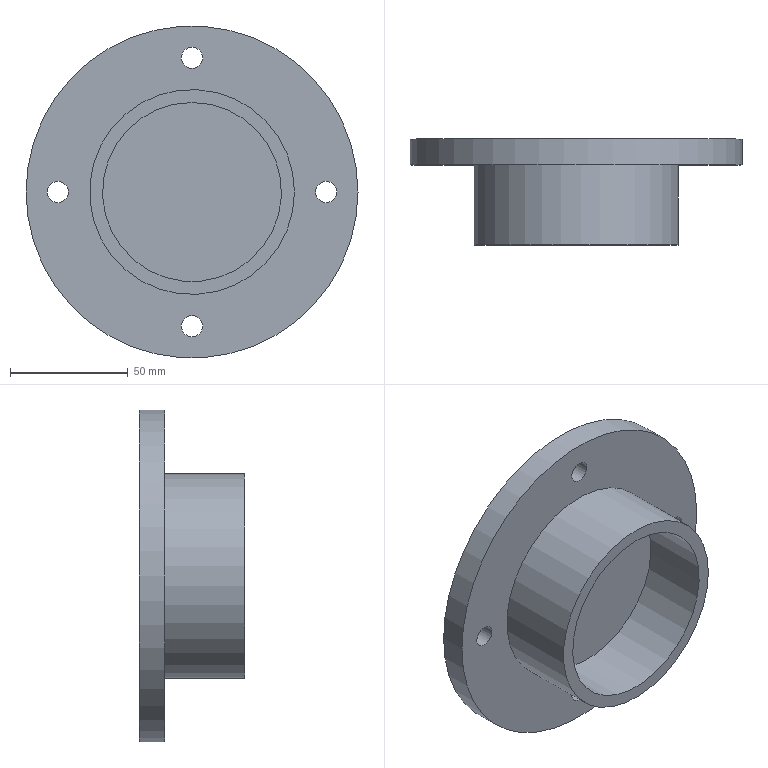Part | NX | features DATUM_CSYS 7, HOLE PACKAGE 7, SIMPLE HOLE 7, SKETCH 6, EXTRACT_DATUM_AXIS 4, EXTRACT_FACE 4, Instance Feature 3, EXTRUDE 2, DELETE FACE 1, Pattern Feature 1 | 1 solid | 13 faces | box 141 x 45 x 141 mm | volume 224063 mm3 | cylinder 8 | plane 5 | commonest cylinder face diameters 9 x4 76 x1 81 x1 87 x1 141 x1
STEP:
#1=CARTESIAN_POINT('',(70.5,-11.,0.));
#2=VERTEX_POINT('',#1);
#3=CARTESIAN_POINT('',(0.,-11.,0.));
#4=DIRECTION('',(0.,-1.,0.));
#5=DIRECTION('',(1.,0.,0.));
#6=AXIS2_PLACEMENT_3D('',#3,#4,#5);
#7=CIRCLE('',#6,70.5);
#8=EDGE_CURVE('',#2,#2,#7,.T.);
#9=ORIENTED_EDGE('',*,*,#8,.F.);
#10=EDGE_LOOP('',(#9));
#11=FACE_BOUND('',#10,.T.);
#12=CARTESIAN_POINT('',(70.5,0.,0.));
#13=VERTEX_POINT('',#12);
#14=CARTESIAN_POINT('',(0.,0.,0.));
#15=DIRECTION('',(0.,-1.,0.));
#16=DIRECTION('',(1.,0.,0.));
#17=AXIS2_PLACEMENT_3D('',#14,#15,#16);
#18=CIRCLE('',#17,70.5);
#19=EDGE_CURVE('',#13,#13,#18,.T.);
#20=ORIENTED_EDGE('',*,*,#19,.T.);
#21=EDGE_LOOP('',(#20));
#22=FACE_BOUND('',#21,.T.);
#23=CARTESIAN_POINT('',(0.,-11.,0.));
#24=DIRECTION('',(0.,1.,0.));
#25=DIRECTION('',(0.,0.,1.));
#26=AXIS2_PLACEMENT_3D('',#23,#24,#25);
#27=CYLINDRICAL_SURFACE('',#26,70.5);
#28=ADVANCED_FACE('',(#11,#22),#27,.T.);
#29=CARTESIAN_POINT('',(0.,-11.,-61.5));
#30=VERTEX_POINT('',#29);
#31=CARTESIAN_POINT('',(0.,-11.,-57.));
#32=DIRECTION('',(0.,-1.,0.));
#33=DIRECTION('',(0.,0.,-1.));
#34=AXIS2_PLACEMENT_3D('',#31,#32,#33);
#35=CIRCLE('',#34,4.5);
#36=EDGE_CURVE('',#30,#30,#35,.T.);
#37=ORIENTED_EDGE('',*,*,#36,.F.);
#38=EDGE_LOOP('',(#37));
#39=FACE_BOUND('',#38,.T.);
#40=CARTESIAN_POINT('',(57.,-11.,-4.5));
#41=VERTEX_POINT('',#40);
#42=CARTESIAN_POINT('',(57.,-11.,0.));
#43=DIRECTION('',(0.,-1.,0.));
#44=DIRECTION('',(0.,0.,-1.));
#45=AXIS2_PLACEMENT_3D('',#42,#43,#44);
#46=CIRCLE('',#45,4.5);
#47=EDGE_CURVE('',#41,#41,#46,.T.);
#48=ORIENTED_EDGE('',*,*,#47,.F.);
#49=EDGE_LOOP('',(#48));
#50=FACE_BOUND('',#49,.T.);
#51=CARTESIAN_POINT('',(0.,-11.,52.5));
#52=VERTEX_POINT('',#51);
#53=CARTESIAN_POINT('',(0.,-11.,57.));
#54=DIRECTION('',(0.,-1.,0.));
#55=DIRECTION('',(0.,0.,-1.));
#56=AXIS2_PLACEMENT_3D('',#53,#54,#55);
#57=CIRCLE('',#56,4.5);
#58=EDGE_CURVE('',#52,#52,#57,.T.);
#59=ORIENTED_EDGE('',*,*,#58,.F.);
#60=EDGE_LOOP('',(#59));
#61=FACE_BOUND('',#60,.T.);
#62=CARTESIAN_POINT('',(-57.,-11.,-4.5));
#63=VERTEX_POINT('',#62);
#64=CARTESIAN_POINT('',(-57.,-11.,0.));
#65=DIRECTION('',(0.,-1.,0.));
#66=DIRECTION('',(0.,0.,-1.));
#67=AXIS2_PLACEMENT_3D('',#64,#65,#66);
#68=CIRCLE('',#67,4.5);
#69=EDGE_CURVE('',#63,#63,#68,.T.);
#70=ORIENTED_EDGE('',*,*,#69,.F.);
#71=EDGE_LOOP('',(#70));
#72=FACE_BOUND('',#71,.T.);
#73=CARTESIAN_POINT('',(43.5,-11.,0.));
#74=VERTEX_POINT('',#73);
#75=CARTESIAN_POINT('',(0.,-11.,0.));
#76=DIRECTION('',(0.,-1.,0.));
#77=DIRECTION('',(1.,0.,0.));
#78=AXIS2_PLACEMENT_3D('',#75,#76,#77);
#79=CIRCLE('',#78,43.5);
#80=EDGE_CURVE('',#74,#74,#79,.T.);
#81=ORIENTED_EDGE('',*,*,#80,.F.);
#82=EDGE_LOOP('',(#81));
#83=FACE_BOUND('',#82,.T.);
#84=ORIENTED_EDGE('',*,*,#8,.T.);
#85=EDGE_LOOP('',(#84));
#86=FACE_BOUND('',#85,.T.);
#87=CARTESIAN_POINT('',(0.,-11.,0.));
#88=DIRECTION('',(0.,-1.,0.));
#89=DIRECTION('',(0.,0.,-1.));
#90=AXIS2_PLACEMENT_3D('',#87,#88,#89);
#91=PLANE('',#90);
#92=ADVANCED_FACE('',(#39,#50,#61,#72,#83,#86),#91,.T.);
#93=CARTESIAN_POINT('',(0.,0.,-61.5));
#94=VERTEX_POINT('',#93);
#95=CARTESIAN_POINT('',(0.,0.,-57.));
#96=DIRECTION('',(0.,-1.,0.));
#97=DIRECTION('',(0.,0.,-1.));
#98=AXIS2_PLACEMENT_3D('',#95,#96,#97);
#99=CIRCLE('',#98,4.5);
#100=EDGE_CURVE('',#94,#94,#99,.T.);
#101=ORIENTED_EDGE('',*,*,#100,.T.);
#102=EDGE_LOOP('',(#101));
#103=FACE_BOUND('',#102,.T.);
#104=CARTESIAN_POINT('',(57.,0.,-4.5));
#105=VERTEX_POINT('',#104);
#106=CARTESIAN_POINT('',(57.,0.,0.));
#107=DIRECTION('',(0.,-1.,0.));
#108=DIRECTION('',(0.,0.,-1.));
#109=AXIS2_PLACEMENT_3D('',#106,#107,#108);
#110=CIRCLE('',#109,4.5);
#111=EDGE_CURVE('',#105,#105,#110,.T.);
#112=ORIENTED_EDGE('',*,*,#111,.T.);
#113=EDGE_LOOP('',(#112));
#114=FACE_BOUND('',#113,.T.);
#115=CARTESIAN_POINT('',(0.,0.,52.5));
#116=VERTEX_POINT('',#115);
#117=CARTESIAN_POINT('',(0.,0.,57.));
#118=DIRECTION('',(0.,-1.,0.));
#119=DIRECTION('',(0.,0.,-1.));
#120=AXIS2_PLACEMENT_3D('',#117,#118,#119);
#121=CIRCLE('',#120,4.5);
#122=EDGE_CURVE('',#116,#116,#121,.T.);
#123=ORIENTED_EDGE('',*,*,#122,.T.);
#124=EDGE_LOOP('',(#123));
#125=FACE_BOUND('',#124,.T.);
#126=CARTESIAN_POINT('',(-57.,0.,-4.5));
#127=VERTEX_POINT('',#126);
#128=CARTESIAN_POINT('',(-57.,0.,0.));
#129=DIRECTION('',(0.,-1.,0.));
#130=DIRECTION('',(0.,0.,-1.));
#131=AXIS2_PLACEMENT_3D('',#128,#129,#130);
#132=CIRCLE('',#131,4.5);
#133=EDGE_CURVE('',#127,#127,#132,.T.);
#134=ORIENTED_EDGE('',*,*,#133,.T.);
#135=EDGE_LOOP('',(#134));
#136=FACE_BOUND('',#135,.T.);
#137=CARTESIAN_POINT('',(0.,0.,-40.5));
#138=VERTEX_POINT('',#137);
#139=CARTESIAN_POINT('',(0.,0.,0.));
#140=DIRECTION('',(0.,-1.,0.));
#141=DIRECTION('',(0.,0.,-1.));
#142=AXIS2_PLACEMENT_3D('',#139,#140,#141);
#143=CIRCLE('',#142,40.5);
#144=EDGE_CURVE('',#138,#138,#143,.T.);
#145=ORIENTED_EDGE('',*,*,#144,.T.);
#146=EDGE_LOOP('',(#145));
#147=FACE_BOUND('',#146,.T.);
#148=ORIENTED_EDGE('',*,*,#19,.F.);
#149=EDGE_LOOP('',(#148));
#150=FACE_BOUND('',#149,.T.);
#151=CARTESIAN_POINT('',(0.,0.,0.));
#152=DIRECTION('',(0.,-1.,0.));
#153=DIRECTION('',(0.,0.,-1.));
#154=AXIS2_PLACEMENT_3D('',#151,#152,#153);
#155=PLANE('',#154);
#156=ADVANCED_FACE('',(#103,#114,#125,#136,#147,#150),#155,.F.);
#157=CARTESIAN_POINT('',(43.5,-45.,0.));
#158=VERTEX_POINT('',#157);
#159=CARTESIAN_POINT('',(0.,-45.,0.));
#160=DIRECTION('',(0.,-1.,0.));
#161=DIRECTION('',(1.,0.,0.));
#162=AXIS2_PLACEMENT_3D('',#159,#160,#161);
#163=CIRCLE('',#162,43.5);
#164=EDGE_CURVE('',#158,#158,#163,.T.);
#165=ORIENTED_EDGE('',*,*,#164,.F.);
#166=EDGE_LOOP('',(#165));
#167=FACE_BOUND('',#166,.T.);
#168=ORIENTED_EDGE('',*,*,#80,.T.);
#169=EDGE_LOOP('',(#168));
#170=FACE_BOUND('',#169,.T.);
#171=CARTESIAN_POINT('',(0.,-45.,0.));
#172=DIRECTION('',(0.,1.,0.));
#173=DIRECTION('',(0.,0.,1.));
#174=AXIS2_PLACEMENT_3D('',#171,#172,#173);
#175=CYLINDRICAL_SURFACE('',#174,43.5);
#176=ADVANCED_FACE('',(#167,#170),#175,.T.);
#177=CARTESIAN_POINT('',(0.,-45.,38.));
#178=VERTEX_POINT('',#177);
#179=CARTESIAN_POINT('',(0.,-45.,0.));
#180=DIRECTION('',(0.,1.,0.));
#181=DIRECTION('',(0.,0.,1.));
#182=AXIS2_PLACEMENT_3D('',#179,#180,#181);
#183=CIRCLE('',#182,38.);
#184=EDGE_CURVE('',#178,#178,#183,.T.);
#185=ORIENTED_EDGE('',*,*,#184,.T.);
#186=EDGE_LOOP('',(#185));
#187=FACE_BOUND('',#186,.T.);
#188=ORIENTED_EDGE('',*,*,#164,.T.);
#189=EDGE_LOOP('',(#188));
#190=FACE_BOUND('',#189,.T.);
#191=CARTESIAN_POINT('',(0.,-45.,0.));
#192=DIRECTION('',(0.,-1.,0.));
#193=DIRECTION('',(0.,0.,-1.));
#194=AXIS2_PLACEMENT_3D('',#191,#192,#193);
#195=PLANE('',#194);
#196=ADVANCED_FACE('',(#187,#190),#195,.T.);
#197=CARTESIAN_POINT('',(0.,-16.,38.));
#198=VERTEX_POINT('',#197);
#199=CARTESIAN_POINT('',(0.,-16.,0.));
#200=DIRECTION('',(0.,1.,0.));
#201=DIRECTION('',(0.,0.,1.));
#202=AXIS2_PLACEMENT_3D('',#199,#200,#201);
#203=CIRCLE('',#202,38.);
#204=EDGE_CURVE('',#198,#198,#203,.F.);
#205=ORIENTED_EDGE('',*,*,#204,.T.);
#206=EDGE_LOOP('',(#205));
#207=FACE_BOUND('',#206,.T.);
#208=CARTESIAN_POINT('',(0.,-16.,0.));
#209=DIRECTION('',(0.,1.,0.));
#210=DIRECTION('',(0.,0.,1.));
#211=AXIS2_PLACEMENT_3D('',#208,#209,#210);
#212=PLANE('',#211);
#213=ADVANCED_FACE('',(#207),#212,.F.);
#214=ORIENTED_EDGE('',*,*,#204,.F.);
#215=EDGE_LOOP('',(#214));
#216=FACE_BOUND('',#215,.T.);
#217=ORIENTED_EDGE('',*,*,#184,.F.);
#218=EDGE_LOOP('',(#217));
#219=FACE_BOUND('',#218,.T.);
#220=CARTESIAN_POINT('',(0.,-45.,0.));
#221=DIRECTION('',(0.,1.,0.));
#222=DIRECTION('',(0.,0.,1.));
#223=AXIS2_PLACEMENT_3D('',#220,#221,#222);
#224=CYLINDRICAL_SURFACE('',#223,38.);
#225=ADVANCED_FACE('',(#216,#219),#224,.F.);
#226=CARTESIAN_POINT('',(0.,-3.,-40.5));
#227=VERTEX_POINT('',#226);
#228=CARTESIAN_POINT('',(0.,-3.,0.));
#229=DIRECTION('',(0.,-1.,0.));
#230=DIRECTION('',(0.,0.,-1.));
#231=AXIS2_PLACEMENT_3D('',#228,#229,#230);
#232=CIRCLE('',#231,40.5);
#233=EDGE_CURVE('',#227,#227,#232,.F.);
#234=ORIENTED_EDGE('',*,*,#233,.T.);
#235=EDGE_LOOP('',(#234));
#236=FACE_BOUND('',#235,.T.);
#237=CARTESIAN_POINT('',(0.,-3.,0.));
#238=DIRECTION('',(0.,-1.,0.));
#239=DIRECTION('',(0.,0.,-1.));
#240=AXIS2_PLACEMENT_3D('',#237,#238,#239);
#241=PLANE('',#240);
#242=ADVANCED_FACE('',(#236),#241,.F.);
#243=ORIENTED_EDGE('',*,*,#233,.F.);
#244=EDGE_LOOP('',(#243));
#245=FACE_BOUND('',#244,.T.);
#246=ORIENTED_EDGE('',*,*,#144,.F.);
#247=EDGE_LOOP('',(#246));
#248=FACE_BOUND('',#247,.T.);
#249=CARTESIAN_POINT('',(0.,0.,0.));
#250=DIRECTION('',(0.,-1.,0.));
#251=DIRECTION('',(0.,0.,-1.));
#252=AXIS2_PLACEMENT_3D('',#249,#250,#251);
#253=CYLINDRICAL_SURFACE('',#252,40.5);
#254=ADVANCED_FACE('',(#245,#248),#253,.F.);
#255=ORIENTED_EDGE('',*,*,#69,.T.);
#256=EDGE_LOOP('',(#255));
#257=FACE_BOUND('',#256,.T.);
#258=ORIENTED_EDGE('',*,*,#133,.F.);
#259=EDGE_LOOP('',(#258));
#260=FACE_BOUND('',#259,.T.);
#261=CARTESIAN_POINT('',(-57.,0.,0.));
#262=DIRECTION('',(0.,-1.,0.));
#263=DIRECTION('',(0.,0.,-1.));
#264=AXIS2_PLACEMENT_3D('',#261,#262,#263);
#265=CYLINDRICAL_SURFACE('',#264,4.5);
#266=ADVANCED_FACE('',(#257,#260),#265,.F.);
#267=ORIENTED_EDGE('',*,*,#58,.T.);
#268=EDGE_LOOP('',(#267));
#269=FACE_BOUND('',#268,.T.);
#270=ORIENTED_EDGE('',*,*,#122,.F.);
#271=EDGE_LOOP('',(#270));
#272=FACE_BOUND('',#271,.T.);
#273=CARTESIAN_POINT('',(0.,0.,57.));
#274=DIRECTION('',(0.,-1.,0.));
#275=DIRECTION('',(0.,0.,-1.));
#276=AXIS2_PLACEMENT_3D('',#273,#274,#275);
#277=CYLINDRICAL_SURFACE('',#276,4.5);
#278=ADVANCED_FACE('',(#269,#272),#277,.F.);
#279=ORIENTED_EDGE('',*,*,#47,.T.);
#280=EDGE_LOOP('',(#279));
#281=FACE_BOUND('',#280,.T.);
#282=ORIENTED_EDGE('',*,*,#111,.F.);
#283=EDGE_LOOP('',(#282));
#284=FACE_BOUND('',#283,.T.);
#285=CARTESIAN_POINT('',(57.,0.,0.));
#286=DIRECTION('',(0.,-1.,0.));
#287=DIRECTION('',(0.,0.,-1.));
#288=AXIS2_PLACEMENT_3D('',#285,#286,#287);
#289=CYLINDRICAL_SURFACE('',#288,4.5);
#290=ADVANCED_FACE('',(#281,#284),#289,.F.);
#291=ORIENTED_EDGE('',*,*,#36,.T.);
#292=EDGE_LOOP('',(#291));
#293=FACE_BOUND('',#292,.T.);
#294=ORIENTED_EDGE('',*,*,#100,.F.);
#295=EDGE_LOOP('',(#294));
#296=FACE_BOUND('',#295,.T.);
#297=CARTESIAN_POINT('',(0.,0.,-57.));
#298=DIRECTION('',(0.,-1.,0.));
#299=DIRECTION('',(0.,0.,-1.));
#300=AXIS2_PLACEMENT_3D('',#297,#298,#299);
#301=CYLINDRICAL_SURFACE('',#300,4.5);
#302=ADVANCED_FACE('',(#293,#296),#301,.F.);
#303=CLOSED_SHELL('',(#28,#92,#156,#176,#196,#213,#225,#242,#254,#266,#278,#290,#302));
#304=MANIFOLD_SOLID_BREP('',#303);
#305=(LENGTH_UNIT()NAMED_UNIT(*)SI_UNIT(.MILLI.,.METRE.));
#306=UNCERTAINTY_MEASURE_WITH_UNIT(LENGTH_MEASURE(0.00001),#305,'','');
#307=(NAMED_UNIT(*)PLANE_ANGLE_UNIT()SI_UNIT($,.RADIAN.));
#308=(NAMED_UNIT(*)SI_UNIT($,.STERADIAN.)SOLID_ANGLE_UNIT());
#309=(GEOMETRIC_REPRESENTATION_CONTEXT(3)GLOBAL_UNCERTAINTY_ASSIGNED_CONTEXT((#306))GLOBAL_UNIT_ASSIGNED_CONTEXT((#305,#307,#308))REPRESENTATION_CONTEXT('',''));
#310=ADVANCED_BREP_SHAPE_REPRESENTATION('',(#304),#309);